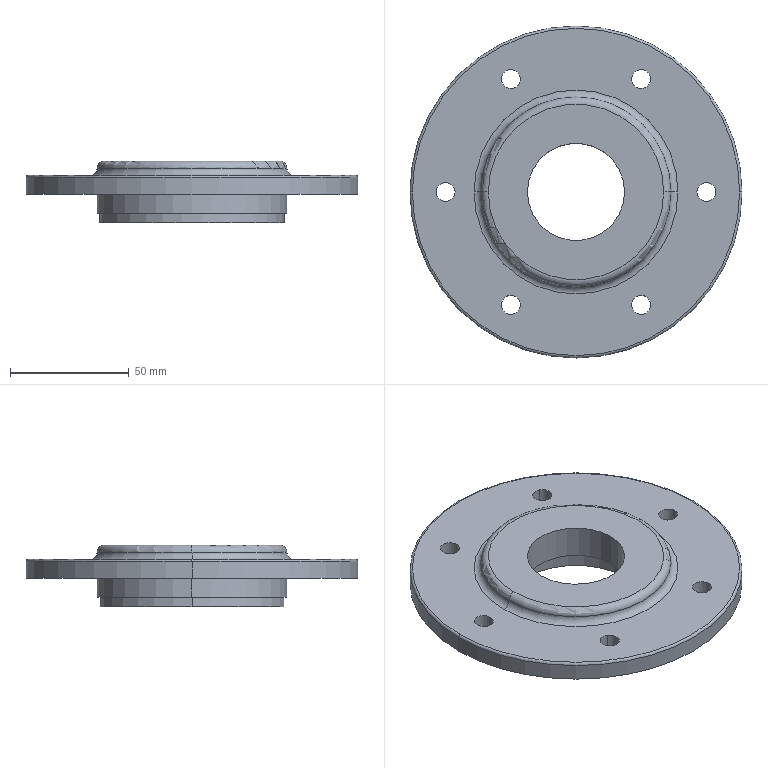Part | SolidWorks | features BaseBody 1 | 1 solid | 34 faces | box 140 x 140 x 26 mm | volume 157732 mm3 | cylinder 22 | torus 6 | plane 6 | commonest cylinder face diameters 8 x12 41 x2 60 x2 78 x2 80 x2 140 x2
STEP:
#1=CARTESIAN_POINT('',(-43.,0.,8.));
#2=VERTEX_POINT('',#1);
#3=CARTESIAN_POINT('',(43.,0.,8.));
#4=VERTEX_POINT('',#3);
#5=CARTESIAN_POINT('',(0.,0.,8.));
#6=DIRECTION('',(0.,0.,1.));
#7=DIRECTION('',(-1.,0.,0.));
#8=AXIS2_PLACEMENT_3D('',#5,#6,#7);
#9=CIRCLE('',#8,43.);
#10=EDGE_CURVE('',#2,#4,#9,.T.);
#11=ORIENTED_EDGE('',*,*,#10,.T.);
#12=CARTESIAN_POINT('',(40.,0.,11.));
#13=VERTEX_POINT('',#12);
#14=CARTESIAN_POINT('',(43.,0.,11.));
#15=DIRECTION('',(0.,1.,0.));
#16=DIRECTION('',(-1.,0.,0.));
#17=AXIS2_PLACEMENT_3D('',#14,#15,#16);
#18=CIRCLE('',#17,3.);
#19=EDGE_CURVE('',#4,#13,#18,.T.);
#20=ORIENTED_EDGE('',*,*,#19,.T.);
#21=CARTESIAN_POINT('',(-40.,0.,11.));
#22=VERTEX_POINT('',#21);
#23=CARTESIAN_POINT('',(0.,0.,11.));
#24=DIRECTION('',(0.,0.,1.));
#25=DIRECTION('',(-1.,0.,0.));
#26=AXIS2_PLACEMENT_3D('',#23,#24,#25);
#27=CIRCLE('',#26,40.);
#28=EDGE_CURVE('',#22,#13,#27,.T.);
#29=ORIENTED_EDGE('',*,*,#28,.F.);
#30=CARTESIAN_POINT('',(-43.,0.,11.));
#31=DIRECTION('',(0.,-1.,0.));
#32=DIRECTION('',(0.,0.,-1.));
#33=AXIS2_PLACEMENT_3D('',#30,#31,#32);
#34=CIRCLE('',#33,3.);
#35=EDGE_CURVE('',#2,#22,#34,.T.);
#36=ORIENTED_EDGE('',*,*,#35,.F.);
#37=EDGE_LOOP('',(#11,#20,#29,#36));
#38=FACE_OUTER_BOUND('',#37,.T.);
#39=CARTESIAN_POINT('',(0.,0.,11.));
#40=DIRECTION('',(0.,0.,-1.));
#41=DIRECTION('',(-1.,0.,0.));
#42=AXIS2_PLACEMENT_3D('',#39,#40,#41);
#43=TOROIDAL_SURFACE('',#42,43.,3.);
#44=ADVANCED_FACE('',(#38),#43,.F.);
#45=CARTESIAN_POINT('',(0.,0.,11.));
#46=DIRECTION('',(0.,0.,1.));
#47=DIRECTION('',(-1.,0.,0.));
#48=AXIS2_PLACEMENT_3D('',#45,#46,#47);
#49=CIRCLE('',#48,40.);
#50=EDGE_CURVE('',#13,#22,#49,.T.);
#51=ORIENTED_EDGE('',*,*,#50,.T.);
#52=CARTESIAN_POINT('',(-37.,0.,14.));
#53=VERTEX_POINT('',#52);
#54=CARTESIAN_POINT('',(-37.,0.,11.));
#55=DIRECTION('',(0.,1.,0.));
#56=DIRECTION('',(-1.,0.,0.));
#57=AXIS2_PLACEMENT_3D('',#54,#55,#56);
#58=CIRCLE('',#57,3.);
#59=EDGE_CURVE('',#22,#53,#58,.T.);
#60=ORIENTED_EDGE('',*,*,#59,.T.);
#61=CARTESIAN_POINT('',(37.,0.,14.));
#62=VERTEX_POINT('',#61);
#63=CARTESIAN_POINT('',(0.,0.,14.));
#64=DIRECTION('',(0.,0.,-1.));
#65=DIRECTION('',(-1.,0.,0.));
#66=AXIS2_PLACEMENT_3D('',#63,#64,#65);
#67=CIRCLE('',#66,37.);
#68=EDGE_CURVE('',#53,#62,#67,.T.);
#69=ORIENTED_EDGE('',*,*,#68,.T.);
#70=CARTESIAN_POINT('',(37.,0.,11.));
#71=DIRECTION('',(0.,-1.,0.));
#72=DIRECTION('',(0.,0.,-1.));
#73=AXIS2_PLACEMENT_3D('',#70,#71,#72);
#74=CIRCLE('',#73,3.);
#75=EDGE_CURVE('',#13,#62,#74,.T.);
#76=ORIENTED_EDGE('',*,*,#75,.F.);
#77=EDGE_LOOP('',(#51,#60,#69,#76));
#78=FACE_OUTER_BOUND('',#77,.T.);
#79=CARTESIAN_POINT('',(0.,0.,11.));
#80=DIRECTION('',(0.,0.,1.));
#81=DIRECTION('',(1.,0.,0.));
#82=AXIS2_PLACEMENT_3D('',#79,#80,#81);
#83=TOROIDAL_SURFACE('',#82,37.,3.);
#84=ADVANCED_FACE('',(#78),#83,.T.);
#85=CARTESIAN_POINT('',(20.5,0.,0.));
#86=VERTEX_POINT('',#85);
#87=CARTESIAN_POINT('',(-20.5,0.,0.));
#88=VERTEX_POINT('',#87);
#89=CARTESIAN_POINT('',(0.,0.,0.));
#90=DIRECTION('',(0.,0.,1.));
#91=DIRECTION('',(-1.,0.,0.));
#92=AXIS2_PLACEMENT_3D('',#89,#90,#91);
#93=CIRCLE('',#92,20.5);
#94=EDGE_CURVE('',#86,#88,#93,.T.);
#95=ORIENTED_EDGE('',*,*,#94,.F.);
#96=CARTESIAN_POINT('',(20.5,0.,14.));
#97=VERTEX_POINT('',#96);
#98=CARTESIAN_POINT('',(20.5,0.,14.));
#99=DIRECTION('',(0.,0.,1.));
#100=VECTOR('',#99,1000.);
#101=LINE('',#98,#100);
#102=EDGE_CURVE('',#86,#97,#101,.T.);
#103=ORIENTED_EDGE('',*,*,#102,.T.);
#104=CARTESIAN_POINT('',(-20.5,0.,14.));
#105=VERTEX_POINT('',#104);
#106=CARTESIAN_POINT('',(0.,0.,14.));
#107=DIRECTION('',(0.,0.,-1.));
#108=DIRECTION('',(-1.,0.,0.));
#109=AXIS2_PLACEMENT_3D('',#106,#107,#108);
#110=CIRCLE('',#109,20.5);
#111=EDGE_CURVE('',#105,#97,#110,.T.);
#112=ORIENTED_EDGE('',*,*,#111,.F.);
#113=CARTESIAN_POINT('',(-20.5,0.,14.));
#114=DIRECTION('',(0.,0.,1.));
#115=VECTOR('',#114,1000.);
#116=LINE('',#113,#115);
#117=EDGE_CURVE('',#88,#105,#116,.T.);
#118=ORIENTED_EDGE('',*,*,#117,.F.);
#119=EDGE_LOOP('',(#95,#103,#112,#118));
#120=FACE_OUTER_BOUND('',#119,.T.);
#121=CARTESIAN_POINT('',(0.,0.,14.));
#122=DIRECTION('',(0.,0.,1.));
#123=DIRECTION('',(-1.,0.,0.));
#124=AXIS2_PLACEMENT_3D('',#121,#122,#123);
#125=CYLINDRICAL_SURFACE('',#124,20.5);
#126=ADVANCED_FACE('',(#120),#125,.F.);
#127=CARTESIAN_POINT('',(-25.5,44.167,0.));
#128=VERTEX_POINT('',#127);
#129=CARTESIAN_POINT('',(-29.5,51.095,0.));
#130=VERTEX_POINT('',#129);
#131=CARTESIAN_POINT('',(-27.5,47.631,0.));
#132=DIRECTION('',(0.,0.,1.));
#133=DIRECTION('',(-0.5,0.866,0.));
#134=AXIS2_PLACEMENT_3D('',#131,#132,#133);
#135=CIRCLE('',#134,4.);
#136=EDGE_CURVE('',#128,#130,#135,.T.);
#137=ORIENTED_EDGE('',*,*,#136,.F.);
#138=CARTESIAN_POINT('',(-25.5,44.167,8.));
#139=VERTEX_POINT('',#138);
#140=CARTESIAN_POINT('',(-25.5,44.167,8.));
#141=DIRECTION('',(0.,0.,1.));
#142=VECTOR('',#141,1000.);
#143=LINE('',#140,#142);
#144=EDGE_CURVE('',#128,#139,#143,.T.);
#145=ORIENTED_EDGE('',*,*,#144,.T.);
#146=CARTESIAN_POINT('',(-29.5,51.095,8.));
#147=VERTEX_POINT('',#146);
#148=CARTESIAN_POINT('',(-27.5,47.631,8.));
#149=DIRECTION('',(0.,0.,-1.));
#150=DIRECTION('',(-0.5,0.866,0.));
#151=AXIS2_PLACEMENT_3D('',#148,#149,#150);
#152=CIRCLE('',#151,4.);
#153=EDGE_CURVE('',#147,#139,#152,.T.);
#154=ORIENTED_EDGE('',*,*,#153,.F.);
#155=CARTESIAN_POINT('',(-29.5,51.095,8.));
#156=DIRECTION('',(0.,0.,1.));
#157=VECTOR('',#156,1000.);
#158=LINE('',#155,#157);
#159=EDGE_CURVE('',#130,#147,#158,.T.);
#160=ORIENTED_EDGE('',*,*,#159,.F.);
#161=EDGE_LOOP('',(#137,#145,#154,#160));
#162=FACE_OUTER_BOUND('',#161,.T.);
#163=CARTESIAN_POINT('',(-27.5,47.631,8.));
#164=DIRECTION('',(0.,0.,1.));
#165=DIRECTION('',(-0.5,0.866,0.));
#166=AXIS2_PLACEMENT_3D('',#163,#164,#165);
#167=CYLINDRICAL_SURFACE('',#166,4.);
#168=ADVANCED_FACE('',(#162),#167,.F.);
#169=CARTESIAN_POINT('',(25.5,44.167,0.));
#170=VERTEX_POINT('',#169);
#171=CARTESIAN_POINT('',(29.5,51.095,0.));
#172=VERTEX_POINT('',#171);
#173=CARTESIAN_POINT('',(27.5,47.631,0.));
#174=DIRECTION('',(0.,0.,1.));
#175=DIRECTION('',(0.5,0.866,0.));
#176=AXIS2_PLACEMENT_3D('',#173,#174,#175);
#177=CIRCLE('',#176,4.);
#178=EDGE_CURVE('',#170,#172,#177,.T.);
#179=ORIENTED_EDGE('',*,*,#178,.F.);
#180=CARTESIAN_POINT('',(25.5,44.167,8.));
#181=VERTEX_POINT('',#180);
#182=CARTESIAN_POINT('',(25.5,44.167,8.));
#183=DIRECTION('',(0.,0.,1.));
#184=VECTOR('',#183,1000.);
#185=LINE('',#182,#184);
#186=EDGE_CURVE('',#170,#181,#185,.T.);
#187=ORIENTED_EDGE('',*,*,#186,.T.);
#188=CARTESIAN_POINT('',(29.5,51.095,8.));
#189=VERTEX_POINT('',#188);
#190=CARTESIAN_POINT('',(27.5,47.631,8.));
#191=DIRECTION('',(0.,0.,-1.));
#192=DIRECTION('',(0.5,0.866,0.));
#193=AXIS2_PLACEMENT_3D('',#190,#191,#192);
#194=CIRCLE('',#193,4.);
#195=EDGE_CURVE('',#189,#181,#194,.T.);
#196=ORIENTED_EDGE('',*,*,#195,.F.);
#197=CARTESIAN_POINT('',(29.5,51.095,8.));
#198=DIRECTION('',(0.,0.,1.));
#199=VECTOR('',#198,1000.);
#200=LINE('',#197,#199);
#201=EDGE_CURVE('',#172,#189,#200,.T.);
#202=ORIENTED_EDGE('',*,*,#201,.F.);
#203=EDGE_LOOP('',(#179,#187,#196,#202));
#204=FACE_OUTER_BOUND('',#203,.T.);
#205=CARTESIAN_POINT('',(27.5,47.631,8.));
#206=DIRECTION('',(0.,0.,1.));
#207=DIRECTION('',(0.5,0.866,0.));
#208=AXIS2_PLACEMENT_3D('',#205,#206,#207);
#209=CYLINDRICAL_SURFACE('',#208,4.);
#210=ADVANCED_FACE('',(#204),#209,.F.);
#211=CARTESIAN_POINT('',(51.,0.,0.));
#212=VERTEX_POINT('',#211);
#213=CARTESIAN_POINT('',(59.,0.,0.));
#214=VERTEX_POINT('',#213);
#215=CARTESIAN_POINT('',(55.,0.,0.));
#216=DIRECTION('',(0.,0.,1.));
#217=DIRECTION('',(1.,0.,0.));
#218=AXIS2_PLACEMENT_3D('',#215,#216,#217);
#219=CIRCLE('',#218,4.);
#220=EDGE_CURVE('',#212,#214,#219,.T.);
#221=ORIENTED_EDGE('',*,*,#220,.F.);
#222=CARTESIAN_POINT('',(51.,0.,8.));
#223=VERTEX_POINT('',#222);
#224=CARTESIAN_POINT('',(51.,0.,8.));
#225=DIRECTION('',(0.,0.,1.));
#226=VECTOR('',#225,1000.);
#227=LINE('',#224,#226);
#228=EDGE_CURVE('',#212,#223,#227,.T.);
#229=ORIENTED_EDGE('',*,*,#228,.T.);
#230=CARTESIAN_POINT('',(59.,0.,8.));
#231=VERTEX_POINT('',#230);
#232=CARTESIAN_POINT('',(55.,0.,8.));
#233=DIRECTION('',(0.,0.,-1.));
#234=DIRECTION('',(1.,0.,0.));
#235=AXIS2_PLACEMENT_3D('',#232,#233,#234);
#236=CIRCLE('',#235,4.);
#237=EDGE_CURVE('',#231,#223,#236,.T.);
#238=ORIENTED_EDGE('',*,*,#237,.F.);
#239=CARTESIAN_POINT('',(59.,0.,8.));
#240=DIRECTION('',(0.,0.,1.));
#241=VECTOR('',#240,1000.);
#242=LINE('',#239,#241);
#243=EDGE_CURVE('',#214,#231,#242,.T.);
#244=ORIENTED_EDGE('',*,*,#243,.F.);
#245=EDGE_LOOP('',(#221,#229,#238,#244));
#246=FACE_OUTER_BOUND('',#245,.T.);
#247=CARTESIAN_POINT('',(55.,0.,8.));
#248=DIRECTION('',(0.,0.,1.));
#249=DIRECTION('',(1.,0.,0.));
#250=AXIS2_PLACEMENT_3D('',#247,#248,#249);
#251=CYLINDRICAL_SURFACE('',#250,4.);
#252=ADVANCED_FACE('',(#246),#251,.F.);
#253=CARTESIAN_POINT('',(25.5,-44.167,0.));
#254=VERTEX_POINT('',#253);
#255=CARTESIAN_POINT('',(29.5,-51.095,0.));
#256=VERTEX_POINT('',#255);
#257=CARTESIAN_POINT('',(27.5,-47.631,0.));
#258=DIRECTION('',(0.,0.,1.));
#259=DIRECTION('',(0.5,-0.866,0.));
#260=AXIS2_PLACEMENT_3D('',#257,#258,#259);
#261=CIRCLE('',#260,4.);
#262=EDGE_CURVE('',#254,#256,#261,.T.);
#263=ORIENTED_EDGE('',*,*,#262,.F.);
#264=CARTESIAN_POINT('',(25.5,-44.167,8.));
#265=VERTEX_POINT('',#264);
#266=CARTESIAN_POINT('',(25.5,-44.167,8.));
#267=DIRECTION('',(0.,0.,1.));
#268=VECTOR('',#267,1000.);
#269=LINE('',#266,#268);
#270=EDGE_CURVE('',#254,#265,#269,.T.);
#271=ORIENTED_EDGE('',*,*,#270,.T.);
#272=CARTESIAN_POINT('',(29.5,-51.095,8.));
#273=VERTEX_POINT('',#272);
#274=CARTESIAN_POINT('',(27.5,-47.631,8.));
#275=DIRECTION('',(0.,0.,-1.));
#276=DIRECTION('',(0.5,-0.866,0.));
#277=AXIS2_PLACEMENT_3D('',#274,#275,#276);
#278=CIRCLE('',#277,4.);
#279=EDGE_CURVE('',#273,#265,#278,.T.);
#280=ORIENTED_EDGE('',*,*,#279,.F.);
#281=CARTESIAN_POINT('',(29.5,-51.095,8.));
#282=DIRECTION('',(0.,0.,1.));
#283=VECTOR('',#282,1000.);
#284=LINE('',#281,#283);
#285=EDGE_CURVE('',#256,#273,#284,.T.);
#286=ORIENTED_EDGE('',*,*,#285,.F.);
#287=EDGE_LOOP('',(#263,#271,#280,#286));
#288=FACE_OUTER_BOUND('',#287,.T.);
#289=CARTESIAN_POINT('',(27.5,-47.631,8.));
#290=DIRECTION('',(0.,0.,1.));
#291=DIRECTION('',(0.5,-0.866,0.));
#292=AXIS2_PLACEMENT_3D('',#289,#290,#291);
#293=CYLINDRICAL_SURFACE('',#292,4.);
#294=ADVANCED_FACE('',(#288),#293,.F.);
#295=CARTESIAN_POINT('',(-25.5,-44.167,0.));
#296=VERTEX_POINT('',#295);
#297=CARTESIAN_POINT('',(-29.5,-51.095,0.));
#298=VERTEX_POINT('',#297);
#299=CARTESIAN_POINT('',(-27.5,-47.631,0.));
#300=DIRECTION('',(0.,0.,1.));
#301=DIRECTION('',(-0.5,-0.866,0.));
#302=AXIS2_PLACEMENT_3D('',#299,#300,#301);
#303=CIRCLE('',#302,4.);
#304=EDGE_CURVE('',#296,#298,#303,.T.);
#305=ORIENTED_EDGE('',*,*,#304,.F.);
#306=CARTESIAN_POINT('',(-25.5,-44.167,8.));
#307=VERTEX_POINT('',#306);
#308=CARTESIAN_POINT('',(-25.5,-44.167,8.));
#309=DIRECTION('',(0.,0.,1.));
#310=VECTOR('',#309,1000.);
#311=LINE('',#308,#310);
#312=EDGE_CURVE('',#296,#307,#311,.T.);
#313=ORIENTED_EDGE('',*,*,#312,.T.);
#314=CARTESIAN_POINT('',(-29.5,-51.095,8.));
#315=VERTEX_POINT('',#314);
#316=CARTESIAN_POINT('',(-27.5,-47.631,8.));
#317=DIRECTION('',(0.,0.,-1.));
#318=DIRECTION('',(-0.5,-0.866,0.));
#319=AXIS2_PLACEMENT_3D('',#316,#317,#318);
#320=CIRCLE('',#319,4.);
#321=EDGE_CURVE('',#315,#307,#320,.T.);
#322=ORIENTED_EDGE('',*,*,#321,.F.);
#323=CARTESIAN_POINT('',(-29.5,-51.095,8.));
#324=DIRECTION('',(0.,0.,1.));
#325=VECTOR('',#324,1000.);
#326=LINE('',#323,#325);
#327=EDGE_CURVE('',#298,#315,#326,.T.);
#328=ORIENTED_EDGE('',*,*,#327,.F.);
#329=EDGE_LOOP('',(#305,#313,#322,#328));
#330=FACE_OUTER_BOUND('',#329,.T.);
#331=CARTESIAN_POINT('',(-27.5,-47.631,8.));
#332=DIRECTION('',(0.,0.,1.));
#333=DIRECTION('',(-0.5,-0.866,0.));
#334=AXIS2_PLACEMENT_3D('',#331,#332,#333);
#335=CYLINDRICAL_SURFACE('',#334,4.);
#336=ADVANCED_FACE('',(#330),#335,.F.);
#337=CARTESIAN_POINT('',(-51.,0.,0.));
#338=VERTEX_POINT('',#337);
#339=CARTESIAN_POINT('',(-59.,0.,0.));
#340=VERTEX_POINT('',#339);
#341=CARTESIAN_POINT('',(-55.,0.,0.));
#342=DIRECTION('',(0.,0.,1.));
#343=DIRECTION('',(-1.,0.,0.));
#344=AXIS2_PLACEMENT_3D('',#341,#342,#343);
#345=CIRCLE('',#344,4.);
#346=EDGE_CURVE('',#338,#340,#345,.T.);
#347=ORIENTED_EDGE('',*,*,#346,.F.);
#348=CARTESIAN_POINT('',(-51.,0.,8.));
#349=VERTEX_POINT('',#348);
#350=CARTESIAN_POINT('',(-51.,0.,8.));
#351=DIRECTION('',(0.,0.,1.));
#352=VECTOR('',#351,1000.);
#353=LINE('',#350,#352);
#354=EDGE_CURVE('',#338,#349,#353,.T.);
#355=ORIENTED_EDGE('',*,*,#354,.T.);
#356=CARTESIAN_POINT('',(-59.,0.,8.));
#357=VERTEX_POINT('',#356);
#358=CARTESIAN_POINT('',(-55.,0.,8.));
#359=DIRECTION('',(0.,0.,-1.));
#360=DIRECTION('',(-1.,0.,0.));
#361=AXIS2_PLACEMENT_3D('',#358,#359,#360);
#362=CIRCLE('',#361,4.);
#363=EDGE_CURVE('',#357,#349,#362,.T.);
#364=ORIENTED_EDGE('',*,*,#363,.F.);
#365=CARTESIAN_POINT('',(-59.,0.,8.));
#366=DIRECTION('',(0.,0.,1.));
#367=VECTOR('',#366,1000.);
#368=LINE('',#365,#367);
#369=EDGE_CURVE('',#340,#357,#368,.T.);
#370=ORIENTED_EDGE('',*,*,#369,.F.);
#371=EDGE_LOOP('',(#347,#355,#364,#370));
#372=FACE_OUTER_BOUND('',#371,.T.);
#373=CARTESIAN_POINT('',(-55.,0.,8.));
#374=DIRECTION('',(0.,0.,1.));
#375=DIRECTION('',(-1.,0.,0.));
#376=AXIS2_PLACEMENT_3D('',#373,#374,#375);
#377=CYLINDRICAL_SURFACE('',#376,4.);
#378=ADVANCED_FACE('',(#372),#377,.F.);
#379=CARTESIAN_POINT('',(70.,0.,7.));
#380=VERTEX_POINT('',#379);
#381=CARTESIAN_POINT('',(-70.,0.,7.));
#382=VERTEX_POINT('',#381);
#383=CARTESIAN_POINT('',(0.,0.,7.));
#384=DIRECTION('',(0.,0.,1.));
#385=DIRECTION('',(-1.,0.,0.));
#386=AXIS2_PLACEMENT_3D('',#383,#384,#385);
#387=CIRCLE('',#386,70.);
#388=EDGE_CURVE('',#380,#382,#387,.T.);
#389=ORIENTED_EDGE('',*,*,#388,.T.);
#390=CARTESIAN_POINT('',(-69.,0.,8.));
#391=VERTEX_POINT('',#390);
#392=CARTESIAN_POINT('',(-69.,0.,7.));
#393=DIRECTION('',(0.,1.,0.));
#394=DIRECTION('',(-1.,0.,0.));
#395=AXIS2_PLACEMENT_3D('',#392,#393,#394);
#396=CIRCLE('',#395,1.);
#397=EDGE_CURVE('',#382,#391,#396,.T.);
#398=ORIENTED_EDGE('',*,*,#397,.T.);
#399=CARTESIAN_POINT('',(69.,0.,8.));
#400=VERTEX_POINT('',#399);
#401=CARTESIAN_POINT('',(0.,0.,8.));
#402=DIRECTION('',(0.,0.,-1.));
#403=DIRECTION('',(-1.,0.,0.));
#404=AXIS2_PLACEMENT_3D('',#401,#402,#403);
#405=CIRCLE('',#404,69.);
#406=EDGE_CURVE('',#391,#400,#405,.T.);
#407=ORIENTED_EDGE('',*,*,#406,.T.);
#408=CARTESIAN_POINT('',(69.,0.,7.));
#409=DIRECTION('',(0.,-1.,0.));
#410=DIRECTION('',(0.,0.,-1.));
#411=AXIS2_PLACEMENT_3D('',#408,#409,#410);
#412=CIRCLE('',#411,1.);
#413=EDGE_CURVE('',#380,#400,#412,.T.);
#414=ORIENTED_EDGE('',*,*,#413,.F.);
#415=EDGE_LOOP('',(#389,#398,#407,#414));
#416=FACE_OUTER_BOUND('',#415,.T.);
#417=CARTESIAN_POINT('',(0.,0.,7.));
#418=DIRECTION('',(0.,0.,1.));
#419=DIRECTION('',(1.,0.,0.));
#420=AXIS2_PLACEMENT_3D('',#417,#418,#419);
#421=TOROIDAL_SURFACE('',#420,69.,1.);
#422=ADVANCED_FACE('',(#416),#421,.T.);
#423=ORIENTED_EDGE('',*,*,#388,.F.);
#424=CARTESIAN_POINT('',(70.,0.,0.));
#425=VERTEX_POINT('',#424);
#426=CARTESIAN_POINT('',(70.,0.,0.));
#427=DIRECTION('',(0.,0.,-1.));
#428=VECTOR('',#427,1000.);
#429=LINE('',#426,#428);
#430=EDGE_CURVE('',#380,#425,#429,.T.);
#431=ORIENTED_EDGE('',*,*,#430,.T.);
#432=CARTESIAN_POINT('',(-70.,0.,0.));
#433=VERTEX_POINT('',#432);
#434=CARTESIAN_POINT('',(0.,0.,0.));
#435=DIRECTION('',(0.,0.,-1.));
#436=DIRECTION('',(-1.,0.,0.));
#437=AXIS2_PLACEMENT_3D('',#434,#435,#436);
#438=CIRCLE('',#437,70.);
#439=EDGE_CURVE('',#433,#425,#438,.T.);
#440=ORIENTED_EDGE('',*,*,#439,.F.);
#441=CARTESIAN_POINT('',(-70.,0.,0.));
#442=DIRECTION('',(0.,0.,-1.));
#443=VECTOR('',#442,1000.);
#444=LINE('',#441,#443);
#445=EDGE_CURVE('',#382,#433,#444,.T.);
#446=ORIENTED_EDGE('',*,*,#445,.F.);
#447=EDGE_LOOP('',(#423,#431,#440,#446));
#448=FACE_OUTER_BOUND('',#447,.T.);
#449=CARTESIAN_POINT('',(0.,0.,0.));
#450=DIRECTION('',(0.,0.,-1.));
#451=DIRECTION('',(-1.,0.,0.));
#452=AXIS2_PLACEMENT_3D('',#449,#450,#451);
#453=CYLINDRICAL_SURFACE('',#452,70.);
#454=ADVANCED_FACE('',(#448),#453,.T.);
#455=CARTESIAN_POINT('',(39.,0.,-8.));
#456=VERTEX_POINT('',#455);
#457=CARTESIAN_POINT('',(-39.,0.,-8.));
#458=VERTEX_POINT('',#457);
#459=CARTESIAN_POINT('',(0.,0.,-8.));
#460=DIRECTION('',(0.,0.,-1.));
#461=DIRECTION('',(1.,0.,0.));
#462=AXIS2_PLACEMENT_3D('',#459,#460,#461);
#463=CIRCLE('',#462,39.);
#464=EDGE_CURVE('',#456,#458,#463,.T.);
#465=ORIENTED_EDGE('',*,*,#464,.T.);
#466=CARTESIAN_POINT('',(-39.,0.,-12.));
#467=VERTEX_POINT('',#466);
#468=CARTESIAN_POINT('',(-39.,0.,-12.));
#469=DIRECTION('',(0.,0.,-1.));
#470=VECTOR('',#469,1000.);
#471=LINE('',#468,#470);
#472=EDGE_CURVE('',#458,#467,#471,.T.);
#473=ORIENTED_EDGE('',*,*,#472,.T.);
#474=CARTESIAN_POINT('',(39.,0.,-12.));
#475=VERTEX_POINT('',#474);
#476=CARTESIAN_POINT('',(0.,0.,-12.));
#477=DIRECTION('',(0.,0.,-1.));
#478=DIRECTION('',(1.,0.,0.));
#479=AXIS2_PLACEMENT_3D('',#476,#477,#478);
#480=CIRCLE('',#479,39.);
#481=EDGE_CURVE('',#475,#467,#480,.T.);
#482=ORIENTED_EDGE('',*,*,#481,.F.);
#483=CARTESIAN_POINT('',(39.,0.,-12.));
#484=DIRECTION('',(0.,0.,-1.));
#485=VECTOR('',#484,1000.);
#486=LINE('',#483,#485);
#487=EDGE_CURVE('',#456,#475,#486,.T.);
#488=ORIENTED_EDGE('',*,*,#487,.F.);
#489=EDGE_LOOP('',(#465,#473,#482,#488));
#490=FACE_OUTER_BOUND('',#489,.T.);
#491=CARTESIAN_POINT('',(0.,0.,-12.));
#492=DIRECTION('',(0.,0.,-1.));
#493=DIRECTION('',(1.,0.,0.));
#494=AXIS2_PLACEMENT_3D('',#491,#492,#493);
#495=CYLINDRICAL_SURFACE('',#494,39.);
#496=ADVANCED_FACE('',(#490),#495,.T.);
#497=CARTESIAN_POINT('',(-30.,0.,-12.));
#498=VERTEX_POINT('',#497);
#499=CARTESIAN_POINT('',(30.,0.,-12.));
#500=VERTEX_POINT('',#499);
#501=CARTESIAN_POINT('',(0.,0.,-12.));
#502=DIRECTION('',(0.,0.,1.));
#503=DIRECTION('',(1.,0.,0.));
#504=AXIS2_PLACEMENT_3D('',#501,#502,#503);
#505=CIRCLE('',#504,30.);
#506=EDGE_CURVE('',#498,#500,#505,.T.);
#507=ORIENTED_EDGE('',*,*,#506,.F.);
#508=CARTESIAN_POINT('',(-30.,0.,0.));
#509=VERTEX_POINT('',#508);
#510=CARTESIAN_POINT('',(-30.,0.,0.));
#511=DIRECTION('',(0.,0.,1.));
#512=VECTOR('',#511,1000.);
#513=LINE('',#510,#512);
#514=EDGE_CURVE('',#498,#509,#513,.T.);
#515=ORIENTED_EDGE('',*,*,#514,.T.);
#516=CARTESIAN_POINT('',(30.,0.,0.));
#517=VERTEX_POINT('',#516);
#518=CARTESIAN_POINT('',(0.,0.,0.));
#519=DIRECTION('',(0.,0.,-1.));
#520=DIRECTION('',(1.,0.,0.));
#521=AXIS2_PLACEMENT_3D('',#518,#519,#520);
#522=CIRCLE('',#521,30.);
#523=EDGE_CURVE('',#517,#509,#522,.T.);
#524=ORIENTED_EDGE('',*,*,#523,.F.);
#525=CARTESIAN_POINT('',(30.,0.,0.));
#526=DIRECTION('',(0.,0.,1.));
#527=VECTOR('',#526,1000.);
#528=LINE('',#525,#527);
#529=EDGE_CURVE('',#500,#517,#528,.T.);
#530=ORIENTED_EDGE('',*,*,#529,.F.);
#531=EDGE_LOOP('',(#507,#515,#524,#530));
#532=FACE_OUTER_BOUND('',#531,.T.);
#533=CARTESIAN_POINT('',(0.,0.,0.));
#534=DIRECTION('',(0.,0.,1.));
#535=DIRECTION('',(1.,0.,0.));
#536=AXIS2_PLACEMENT_3D('',#533,#534,#535);
#537=CYLINDRICAL_SURFACE('',#536,30.);
#538=ADVANCED_FACE('',(#532),#537,.F.);
#539=CARTESIAN_POINT('',(40.,0.,-8.));
#540=VERTEX_POINT('',#539);
#541=CARTESIAN_POINT('',(-40.,0.,-8.));
#542=VERTEX_POINT('',#541);
#543=CARTESIAN_POINT('',(0.,0.,-8.));
#544=DIRECTION('',(0.,0.,1.));
#545=DIRECTION('',(1.,0.,0.));
#546=AXIS2_PLACEMENT_3D('',#543,#544,#545);
#547=CIRCLE('',#546,40.);
#548=EDGE_CURVE('',#540,#542,#547,.T.);
#549=ORIENTED_EDGE('',*,*,#548,.T.);
#550=CARTESIAN_POINT('',(-40.,0.,0.));
#551=VERTEX_POINT('',#550);
#552=CARTESIAN_POINT('',(-40.,0.,0.));
#553=DIRECTION('',(0.,0.,1.));
#554=VECTOR('',#553,1000.);
#555=LINE('',#552,#554);
#556=EDGE_CURVE('',#542,#551,#555,.T.);
#557=ORIENTED_EDGE('',*,*,#556,.T.);
#558=CARTESIAN_POINT('',(40.,0.,0.));
#559=VERTEX_POINT('',#558);
#560=CARTESIAN_POINT('',(0.,0.,0.));
#561=DIRECTION('',(0.,0.,1.));
#562=DIRECTION('',(1.,0.,0.));
#563=AXIS2_PLACEMENT_3D('',#560,#561,#562);
#564=CIRCLE('',#563,40.);
#565=EDGE_CURVE('',#559,#551,#564,.T.);
#566=ORIENTED_EDGE('',*,*,#565,.F.);
#567=CARTESIAN_POINT('',(40.,0.,0.));
#568=DIRECTION('',(0.,0.,1.));
#569=VECTOR('',#568,1000.);
#570=LINE('',#567,#569);
#571=EDGE_CURVE('',#540,#559,#570,.T.);
#572=ORIENTED_EDGE('',*,*,#571,.F.);
#573=EDGE_LOOP('',(#549,#557,#566,#572));
#574=FACE_OUTER_BOUND('',#573,.T.);
#575=CARTESIAN_POINT('',(0.,0.,0.));
#576=DIRECTION('',(0.,0.,1.));
#577=DIRECTION('',(1.,0.,0.));
#578=AXIS2_PLACEMENT_3D('',#575,#576,#577);
#579=CYLINDRICAL_SURFACE('',#578,40.);
#580=ADVANCED_FACE('',(#574),#579,.T.);
#581=ORIENTED_EDGE('',*,*,#363,.T.);
#582=CARTESIAN_POINT('',(-55.,0.,8.));
#583=DIRECTION('',(0.,0.,-1.));
#584=DIRECTION('',(-1.,0.,0.));
#585=AXIS2_PLACEMENT_3D('',#582,#583,#584);
#586=CIRCLE('',#585,4.);
#587=EDGE_CURVE('',#349,#357,#586,.T.);
#588=ORIENTED_EDGE('',*,*,#587,.T.);
#589=EDGE_LOOP('',(#581,#588));
#590=FACE_BOUND('',#589,.T.);
#591=ORIENTED_EDGE('',*,*,#321,.T.);
#592=CARTESIAN_POINT('',(-27.5,-47.631,8.));
#593=DIRECTION('',(0.,0.,-1.));
#594=DIRECTION('',(-0.5,-0.866,0.));
#595=AXIS2_PLACEMENT_3D('',#592,#593,#594);
#596=CIRCLE('',#595,4.);
#597=EDGE_CURVE('',#307,#315,#596,.T.);
#598=ORIENTED_EDGE('',*,*,#597,.T.);
#599=EDGE_LOOP('',(#591,#598));
#600=FACE_BOUND('',#599,.T.);
#601=ORIENTED_EDGE('',*,*,#279,.T.);
#602=CARTESIAN_POINT('',(27.5,-47.631,8.));
#603=DIRECTION('',(0.,0.,-1.));
#604=DIRECTION('',(0.5,-0.866,0.));
#605=AXIS2_PLACEMENT_3D('',#602,#603,#604);
#606=CIRCLE('',#605,4.);
#607=EDGE_CURVE('',#265,#273,#606,.T.);
#608=ORIENTED_EDGE('',*,*,#607,.T.);
#609=EDGE_LOOP('',(#601,#608));
#610=FACE_BOUND('',#609,.T.);
#611=ORIENTED_EDGE('',*,*,#237,.T.);
#612=CARTESIAN_POINT('',(55.,0.,8.));
#613=DIRECTION('',(0.,0.,-1.));
#614=DIRECTION('',(1.,0.,0.));
#615=AXIS2_PLACEMENT_3D('',#612,#613,#614);
#616=CIRCLE('',#615,4.);
#617=EDGE_CURVE('',#223,#231,#616,.T.);
#618=ORIENTED_EDGE('',*,*,#617,.T.);
#619=EDGE_LOOP('',(#611,#618));
#620=FACE_BOUND('',#619,.T.);
#621=ORIENTED_EDGE('',*,*,#195,.T.);
#622=CARTESIAN_POINT('',(27.5,47.631,8.));
#623=DIRECTION('',(0.,0.,-1.));
#624=DIRECTION('',(0.5,0.866,0.));
#625=AXIS2_PLACEMENT_3D('',#622,#623,#624);
#626=CIRCLE('',#625,4.);
#627=EDGE_CURVE('',#181,#189,#626,.T.);
#628=ORIENTED_EDGE('',*,*,#627,.T.);
#629=EDGE_LOOP('',(#621,#628));
#630=FACE_BOUND('',#629,.T.);
#631=ORIENTED_EDGE('',*,*,#153,.T.);
#632=CARTESIAN_POINT('',(-27.5,47.631,8.));
#633=DIRECTION('',(0.,0.,-1.));
#634=DIRECTION('',(-0.5,0.866,0.));
#635=AXIS2_PLACEMENT_3D('',#632,#633,#634);
#636=CIRCLE('',#635,4.);
#637=EDGE_CURVE('',#139,#147,#636,.T.);
#638=ORIENTED_EDGE('',*,*,#637,.T.);
#639=EDGE_LOOP('',(#631,#638));
#640=FACE_BOUND('',#639,.T.);
#641=ORIENTED_EDGE('',*,*,#10,.F.);
#642=CARTESIAN_POINT('',(0.,0.,8.));
#643=DIRECTION('',(0.,0.,1.));
#644=DIRECTION('',(-1.,0.,0.));
#645=AXIS2_PLACEMENT_3D('',#642,#643,#644);
#646=CIRCLE('',#645,43.);
#647=EDGE_CURVE('',#4,#2,#646,.T.);
#648=ORIENTED_EDGE('',*,*,#647,.F.);
#649=EDGE_LOOP('',(#641,#648));
#650=FACE_BOUND('',#649,.T.);
#651=CARTESIAN_POINT('',(0.,0.,8.));
#652=DIRECTION('',(0.,0.,-1.));
#653=DIRECTION('',(-1.,0.,0.));
#654=AXIS2_PLACEMENT_3D('',#651,#652,#653);
#655=CIRCLE('',#654,69.);
#656=EDGE_CURVE('',#400,#391,#655,.T.);
#657=ORIENTED_EDGE('',*,*,#656,.F.);
#658=ORIENTED_EDGE('',*,*,#406,.F.);
#659=EDGE_LOOP('',(#657,#658));
#660=FACE_OUTER_BOUND('',#659,.T.);
#661=CARTESIAN_POINT('',(0.,0.,8.));
#662=DIRECTION('',(0.,0.,1.));
#663=DIRECTION('',(1.,0.,0.));
#664=AXIS2_PLACEMENT_3D('',#661,#662,#663);
#665=PLANE('',#664);
#666=ADVANCED_FACE('',(#590,#600,#610,#620,#630,#640,#650,#660),#665,.T.);
#667=ORIENTED_EDGE('',*,*,#111,.T.);
#668=CARTESIAN_POINT('',(0.,0.,14.));
#669=DIRECTION('',(0.,0.,-1.));
#670=DIRECTION('',(-1.,0.,0.));
#671=AXIS2_PLACEMENT_3D('',#668,#669,#670);
#672=CIRCLE('',#671,20.5);
#673=EDGE_CURVE('',#97,#105,#672,.T.);
#674=ORIENTED_EDGE('',*,*,#673,.T.);
#675=EDGE_LOOP('',(#667,#674));
#676=FACE_BOUND('',#675,.T.);
#677=CARTESIAN_POINT('',(0.,0.,14.));
#678=DIRECTION('',(0.,0.,-1.));
#679=DIRECTION('',(-1.,0.,0.));
#680=AXIS2_PLACEMENT_3D('',#677,#678,#679);
#681=CIRCLE('',#680,37.);
#682=EDGE_CURVE('',#62,#53,#681,.T.);
#683=ORIENTED_EDGE('',*,*,#682,.F.);
#684=ORIENTED_EDGE('',*,*,#68,.F.);
#685=EDGE_LOOP('',(#683,#684));
#686=FACE_OUTER_BOUND('',#685,.T.);
#687=CARTESIAN_POINT('',(0.,0.,14.));
#688=DIRECTION('',(0.,0.,1.));
#689=DIRECTION('',(1.,0.,0.));
#690=AXIS2_PLACEMENT_3D('',#687,#688,#689);
#691=PLANE('',#690);
#692=ADVANCED_FACE('',(#676,#686),#691,.T.);
#693=ORIENTED_EDGE('',*,*,#464,.F.);
#694=CARTESIAN_POINT('',(0.,0.,-8.));
#695=DIRECTION('',(0.,0.,-1.));
#696=DIRECTION('',(1.,0.,0.));
#697=AXIS2_PLACEMENT_3D('',#694,#695,#696);
#698=CIRCLE('',#697,39.);
#699=EDGE_CURVE('',#458,#456,#698,.T.);
#700=ORIENTED_EDGE('',*,*,#699,.F.);
#701=EDGE_LOOP('',(#693,#700));
#702=FACE_BOUND('',#701,.T.);
#703=ORIENTED_EDGE('',*,*,#548,.F.);
#704=CARTESIAN_POINT('',(0.,0.,-8.));
#705=DIRECTION('',(0.,0.,1.));
#706=DIRECTION('',(1.,0.,0.));
#707=AXIS2_PLACEMENT_3D('',#704,#705,#706);
#708=CIRCLE('',#707,40.);
#709=EDGE_CURVE('',#542,#540,#708,.T.);
#710=ORIENTED_EDGE('',*,*,#709,.F.);
#711=EDGE_LOOP('',(#703,#710));
#712=FACE_OUTER_BOUND('',#711,.T.);
#713=CARTESIAN_POINT('',(0.,0.,-8.));
#714=DIRECTION('',(0.,0.,1.));
#715=DIRECTION('',(1.,0.,0.));
#716=AXIS2_PLACEMENT_3D('',#713,#714,#715);
#717=PLANE('',#716);
#718=ADVANCED_FACE('',(#702,#712),#717,.F.);
#719=CARTESIAN_POINT('',(0.,0.,-12.));
#720=DIRECTION('',(0.,0.,1.));
#721=DIRECTION('',(1.,0.,0.));
#722=AXIS2_PLACEMENT_3D('',#719,#720,#721);
#723=CIRCLE('',#722,30.);
#724=EDGE_CURVE('',#500,#498,#723,.T.);
#725=ORIENTED_EDGE('',*,*,#724,.T.);
#726=ORIENTED_EDGE('',*,*,#506,.T.);
#727=EDGE_LOOP('',(#725,#726));
#728=FACE_BOUND('',#727,.T.);
#729=ORIENTED_EDGE('',*,*,#481,.T.);
#730=CARTESIAN_POINT('',(0.,0.,-12.));
#731=DIRECTION('',(0.,0.,-1.));
#732=DIRECTION('',(1.,0.,0.));
#733=AXIS2_PLACEMENT_3D('',#730,#731,#732);
#734=CIRCLE('',#733,39.);
#735=EDGE_CURVE('',#467,#475,#734,.T.);
#736=ORIENTED_EDGE('',*,*,#735,.T.);
#737=EDGE_LOOP('',(#729,#736));
#738=FACE_OUTER_BOUND('',#737,.T.);
#739=CARTESIAN_POINT('',(0.,0.,-12.));
#740=DIRECTION('',(0.,0.,1.));
#741=DIRECTION('',(1.,0.,0.));
#742=AXIS2_PLACEMENT_3D('',#739,#740,#741);
#743=PLANE('',#742);
#744=ADVANCED_FACE('',(#728,#738),#743,.F.);
#745=CARTESIAN_POINT('',(-27.5,47.631,0.));
#746=DIRECTION('',(0.,0.,1.));
#747=DIRECTION('',(-0.5,0.866,0.));
#748=AXIS2_PLACEMENT_3D('',#745,#746,#747);
#749=CIRCLE('',#748,4.);
#750=EDGE_CURVE('',#130,#128,#749,.T.);
#751=ORIENTED_EDGE('',*,*,#750,.T.);
#752=ORIENTED_EDGE('',*,*,#136,.T.);
#753=EDGE_LOOP('',(#751,#752));
#754=FACE_BOUND('',#753,.T.);
#755=CARTESIAN_POINT('',(27.5,47.631,0.));
#756=DIRECTION('',(0.,0.,1.));
#757=DIRECTION('',(0.5,0.866,0.));
#758=AXIS2_PLACEMENT_3D('',#755,#756,#757);
#759=CIRCLE('',#758,4.);
#760=EDGE_CURVE('',#172,#170,#759,.T.);
#761=ORIENTED_EDGE('',*,*,#760,.T.);
#762=ORIENTED_EDGE('',*,*,#178,.T.);
#763=EDGE_LOOP('',(#761,#762));
#764=FACE_BOUND('',#763,.T.);
#765=CARTESIAN_POINT('',(55.,0.,0.));
#766=DIRECTION('',(0.,0.,1.));
#767=DIRECTION('',(1.,0.,0.));
#768=AXIS2_PLACEMENT_3D('',#765,#766,#767);
#769=CIRCLE('',#768,4.);
#770=EDGE_CURVE('',#214,#212,#769,.T.);
#771=ORIENTED_EDGE('',*,*,#770,.T.);
#772=ORIENTED_EDGE('',*,*,#220,.T.);
#773=EDGE_LOOP('',(#771,#772));
#774=FACE_BOUND('',#773,.T.);
#775=CARTESIAN_POINT('',(27.5,-47.631,0.));
#776=DIRECTION('',(0.,0.,1.));
#777=DIRECTION('',(0.5,-0.866,0.));
#778=AXIS2_PLACEMENT_3D('',#775,#776,#777);
#779=CIRCLE('',#778,4.);
#780=EDGE_CURVE('',#256,#254,#779,.T.);
#781=ORIENTED_EDGE('',*,*,#780,.T.);
#782=ORIENTED_EDGE('',*,*,#262,.T.);
#783=EDGE_LOOP('',(#781,#782));
#784=FACE_BOUND('',#783,.T.);
#785=CARTESIAN_POINT('',(-27.5,-47.631,0.));
#786=DIRECTION('',(0.,0.,1.));
#787=DIRECTION('',(-0.5,-0.866,0.));
#788=AXIS2_PLACEMENT_3D('',#785,#786,#787);
#789=CIRCLE('',#788,4.);
#790=EDGE_CURVE('',#298,#296,#789,.T.);
#791=ORIENTED_EDGE('',*,*,#790,.T.);
#792=ORIENTED_EDGE('',*,*,#304,.T.);
#793=EDGE_LOOP('',(#791,#792));
#794=FACE_BOUND('',#793,.T.);
#795=CARTESIAN_POINT('',(-55.,0.,0.));
#796=DIRECTION('',(0.,0.,1.));
#797=DIRECTION('',(-1.,0.,0.));
#798=AXIS2_PLACEMENT_3D('',#795,#796,#797);
#799=CIRCLE('',#798,4.);
#800=EDGE_CURVE('',#340,#338,#799,.T.);
#801=ORIENTED_EDGE('',*,*,#800,.T.);
#802=ORIENTED_EDGE('',*,*,#346,.T.);
#803=EDGE_LOOP('',(#801,#802));
#804=FACE_BOUND('',#803,.T.);
#805=ORIENTED_EDGE('',*,*,#565,.T.);
#806=CARTESIAN_POINT('',(0.,0.,0.));
#807=DIRECTION('',(0.,0.,1.));
#808=DIRECTION('',(1.,0.,0.));
#809=AXIS2_PLACEMENT_3D('',#806,#807,#808);
#810=CIRCLE('',#809,40.);
#811=EDGE_CURVE('',#551,#559,#810,.T.);
#812=ORIENTED_EDGE('',*,*,#811,.T.);
#813=EDGE_LOOP('',(#805,#812));
#814=FACE_BOUND('',#813,.T.);
#815=ORIENTED_EDGE('',*,*,#439,.T.);
#816=CARTESIAN_POINT('',(0.,0.,0.));
#817=DIRECTION('',(0.,0.,-1.));
#818=DIRECTION('',(-1.,0.,0.));
#819=AXIS2_PLACEMENT_3D('',#816,#817,#818);
#820=CIRCLE('',#819,70.);
#821=EDGE_CURVE('',#425,#433,#820,.T.);
#822=ORIENTED_EDGE('',*,*,#821,.T.);
#823=EDGE_LOOP('',(#815,#822));
#824=FACE_OUTER_BOUND('',#823,.T.);
#825=CARTESIAN_POINT('',(0.,0.,0.));
#826=DIRECTION('',(0.,0.,1.));
#827=DIRECTION('',(1.,0.,0.));
#828=AXIS2_PLACEMENT_3D('',#825,#826,#827);
#829=PLANE('',#828);
#830=ADVANCED_FACE('',(#754,#764,#774,#784,#794,#804,#814,#824),#829,.F.);
#831=CARTESIAN_POINT('',(0.,0.,0.));
#832=DIRECTION('',(0.,0.,1.));
#833=DIRECTION('',(-1.,0.,0.));
#834=AXIS2_PLACEMENT_3D('',#831,#832,#833);
#835=CIRCLE('',#834,20.5);
#836=EDGE_CURVE('',#88,#86,#835,.T.);
#837=ORIENTED_EDGE('',*,*,#836,.T.);
#838=ORIENTED_EDGE('',*,*,#94,.T.);
#839=EDGE_LOOP('',(#837,#838));
#840=FACE_BOUND('',#839,.T.);
#841=ORIENTED_EDGE('',*,*,#523,.T.);
#842=CARTESIAN_POINT('',(0.,0.,0.));
#843=DIRECTION('',(0.,0.,-1.));
#844=DIRECTION('',(1.,0.,0.));
#845=AXIS2_PLACEMENT_3D('',#842,#843,#844);
#846=CIRCLE('',#845,30.);
#847=EDGE_CURVE('',#509,#517,#846,.T.);
#848=ORIENTED_EDGE('',*,*,#847,.T.);
#849=EDGE_LOOP('',(#841,#848));
#850=FACE_OUTER_BOUND('',#849,.T.);
#851=CARTESIAN_POINT('',(0.,0.,0.));
#852=DIRECTION('',(0.,0.,1.));
#853=DIRECTION('',(1.,0.,0.));
#854=AXIS2_PLACEMENT_3D('',#851,#852,#853);
#855=PLANE('',#854);
#856=ADVANCED_FACE('',(#840,#850),#855,.F.);
#857=ORIENTED_EDGE('',*,*,#556,.F.);
#858=ORIENTED_EDGE('',*,*,#709,.T.);
#859=ORIENTED_EDGE('',*,*,#571,.T.);
#860=ORIENTED_EDGE('',*,*,#811,.F.);
#861=EDGE_LOOP('',(#857,#858,#859,#860));
#862=FACE_OUTER_BOUND('',#861,.T.);
#863=CARTESIAN_POINT('',(0.,0.,0.));
#864=DIRECTION('',(0.,0.,1.));
#865=DIRECTION('',(1.,0.,0.));
#866=AXIS2_PLACEMENT_3D('',#863,#864,#865);
#867=CYLINDRICAL_SURFACE('',#866,40.);
#868=ADVANCED_FACE('',(#862),#867,.T.);
#869=ORIENTED_EDGE('',*,*,#514,.F.);
#870=ORIENTED_EDGE('',*,*,#724,.F.);
#871=ORIENTED_EDGE('',*,*,#529,.T.);
#872=ORIENTED_EDGE('',*,*,#847,.F.);
#873=EDGE_LOOP('',(#869,#870,#871,#872));
#874=FACE_OUTER_BOUND('',#873,.T.);
#875=CARTESIAN_POINT('',(0.,0.,0.));
#876=DIRECTION('',(0.,0.,1.));
#877=DIRECTION('',(1.,0.,0.));
#878=AXIS2_PLACEMENT_3D('',#875,#876,#877);
#879=CYLINDRICAL_SURFACE('',#878,30.);
#880=ADVANCED_FACE('',(#874),#879,.F.);
#881=ORIENTED_EDGE('',*,*,#472,.F.);
#882=ORIENTED_EDGE('',*,*,#699,.T.);
#883=ORIENTED_EDGE('',*,*,#487,.T.);
#884=ORIENTED_EDGE('',*,*,#735,.F.);
#885=EDGE_LOOP('',(#881,#882,#883,#884));
#886=FACE_OUTER_BOUND('',#885,.T.);
#887=CARTESIAN_POINT('',(0.,0.,-12.));
#888=DIRECTION('',(0.,0.,-1.));
#889=DIRECTION('',(1.,0.,0.));
#890=AXIS2_PLACEMENT_3D('',#887,#888,#889);
#891=CYLINDRICAL_SURFACE('',#890,39.);
#892=ADVANCED_FACE('',(#886),#891,.T.);
#893=ORIENTED_EDGE('',*,*,#430,.F.);
#894=CARTESIAN_POINT('',(0.,0.,7.));
#895=DIRECTION('',(0.,0.,1.));
#896=DIRECTION('',(-1.,0.,0.));
#897=AXIS2_PLACEMENT_3D('',#894,#895,#896);
#898=CIRCLE('',#897,70.);
#899=EDGE_CURVE('',#382,#380,#898,.T.);
#900=ORIENTED_EDGE('',*,*,#899,.F.);
#901=ORIENTED_EDGE('',*,*,#445,.T.);
#902=ORIENTED_EDGE('',*,*,#821,.F.);
#903=EDGE_LOOP('',(#893,#900,#901,#902));
#904=FACE_OUTER_BOUND('',#903,.T.);
#905=CARTESIAN_POINT('',(0.,0.,0.));
#906=DIRECTION('',(0.,0.,-1.));
#907=DIRECTION('',(-1.,0.,0.));
#908=AXIS2_PLACEMENT_3D('',#905,#906,#907);
#909=CYLINDRICAL_SURFACE('',#908,70.);
#910=ADVANCED_FACE('',(#904),#909,.T.);
#911=ORIENTED_EDGE('',*,*,#397,.F.);
#912=ORIENTED_EDGE('',*,*,#899,.T.);
#913=ORIENTED_EDGE('',*,*,#413,.T.);
#914=ORIENTED_EDGE('',*,*,#656,.T.);
#915=EDGE_LOOP('',(#911,#912,#913,#914));
#916=FACE_OUTER_BOUND('',#915,.T.);
#917=CARTESIAN_POINT('',(0.,0.,7.));
#918=DIRECTION('',(0.,0.,1.));
#919=DIRECTION('',(1.,0.,0.));
#920=AXIS2_PLACEMENT_3D('',#917,#918,#919);
#921=TOROIDAL_SURFACE('',#920,69.,1.);
#922=ADVANCED_FACE('',(#916),#921,.T.);
#923=ORIENTED_EDGE('',*,*,#354,.F.);
#924=ORIENTED_EDGE('',*,*,#800,.F.);
#925=ORIENTED_EDGE('',*,*,#369,.T.);
#926=ORIENTED_EDGE('',*,*,#587,.F.);
#927=EDGE_LOOP('',(#923,#924,#925,#926));
#928=FACE_OUTER_BOUND('',#927,.T.);
#929=CARTESIAN_POINT('',(-55.,0.,8.));
#930=DIRECTION('',(0.,0.,1.));
#931=DIRECTION('',(-1.,0.,0.));
#932=AXIS2_PLACEMENT_3D('',#929,#930,#931);
#933=CYLINDRICAL_SURFACE('',#932,4.);
#934=ADVANCED_FACE('',(#928),#933,.F.);
#935=ORIENTED_EDGE('',*,*,#312,.F.);
#936=ORIENTED_EDGE('',*,*,#790,.F.);
#937=ORIENTED_EDGE('',*,*,#327,.T.);
#938=ORIENTED_EDGE('',*,*,#597,.F.);
#939=EDGE_LOOP('',(#935,#936,#937,#938));
#940=FACE_OUTER_BOUND('',#939,.T.);
#941=CARTESIAN_POINT('',(-27.5,-47.631,8.));
#942=DIRECTION('',(0.,0.,1.));
#943=DIRECTION('',(-0.5,-0.866,0.));
#944=AXIS2_PLACEMENT_3D('',#941,#942,#943);
#945=CYLINDRICAL_SURFACE('',#944,4.);
#946=ADVANCED_FACE('',(#940),#945,.F.);
#947=ORIENTED_EDGE('',*,*,#270,.F.);
#948=ORIENTED_EDGE('',*,*,#780,.F.);
#949=ORIENTED_EDGE('',*,*,#285,.T.);
#950=ORIENTED_EDGE('',*,*,#607,.F.);
#951=EDGE_LOOP('',(#947,#948,#949,#950));
#952=FACE_OUTER_BOUND('',#951,.T.);
#953=CARTESIAN_POINT('',(27.5,-47.631,8.));
#954=DIRECTION('',(0.,0.,1.));
#955=DIRECTION('',(0.5,-0.866,0.));
#956=AXIS2_PLACEMENT_3D('',#953,#954,#955);
#957=CYLINDRICAL_SURFACE('',#956,4.);
#958=ADVANCED_FACE('',(#952),#957,.F.);
#959=ORIENTED_EDGE('',*,*,#228,.F.);
#960=ORIENTED_EDGE('',*,*,#770,.F.);
#961=ORIENTED_EDGE('',*,*,#243,.T.);
#962=ORIENTED_EDGE('',*,*,#617,.F.);
#963=EDGE_LOOP('',(#959,#960,#961,#962));
#964=FACE_OUTER_BOUND('',#963,.T.);
#965=CARTESIAN_POINT('',(55.,0.,8.));
#966=DIRECTION('',(0.,0.,1.));
#967=DIRECTION('',(1.,0.,0.));
#968=AXIS2_PLACEMENT_3D('',#965,#966,#967);
#969=CYLINDRICAL_SURFACE('',#968,4.);
#970=ADVANCED_FACE('',(#964),#969,.F.);
#971=ORIENTED_EDGE('',*,*,#186,.F.);
#972=ORIENTED_EDGE('',*,*,#760,.F.);
#973=ORIENTED_EDGE('',*,*,#201,.T.);
#974=ORIENTED_EDGE('',*,*,#627,.F.);
#975=EDGE_LOOP('',(#971,#972,#973,#974));
#976=FACE_OUTER_BOUND('',#975,.T.);
#977=CARTESIAN_POINT('',(27.5,47.631,8.));
#978=DIRECTION('',(0.,0.,1.));
#979=DIRECTION('',(0.5,0.866,0.));
#980=AXIS2_PLACEMENT_3D('',#977,#978,#979);
#981=CYLINDRICAL_SURFACE('',#980,4.);
#982=ADVANCED_FACE('',(#976),#981,.F.);
#983=ORIENTED_EDGE('',*,*,#144,.F.);
#984=ORIENTED_EDGE('',*,*,#750,.F.);
#985=ORIENTED_EDGE('',*,*,#159,.T.);
#986=ORIENTED_EDGE('',*,*,#637,.F.);
#987=EDGE_LOOP('',(#983,#984,#985,#986));
#988=FACE_OUTER_BOUND('',#987,.T.);
#989=CARTESIAN_POINT('',(-27.5,47.631,8.));
#990=DIRECTION('',(0.,0.,1.));
#991=DIRECTION('',(-0.5,0.866,0.));
#992=AXIS2_PLACEMENT_3D('',#989,#990,#991);
#993=CYLINDRICAL_SURFACE('',#992,4.);
#994=ADVANCED_FACE('',(#988),#993,.F.);
#995=ORIENTED_EDGE('',*,*,#102,.F.);
#996=ORIENTED_EDGE('',*,*,#836,.F.);
#997=ORIENTED_EDGE('',*,*,#117,.T.);
#998=ORIENTED_EDGE('',*,*,#673,.F.);
#999=EDGE_LOOP('',(#995,#996,#997,#998));
#1000=FACE_OUTER_BOUND('',#999,.T.);
#1001=CARTESIAN_POINT('',(0.,0.,14.));
#1002=DIRECTION('',(0.,0.,1.));
#1003=DIRECTION('',(-1.,0.,0.));
#1004=AXIS2_PLACEMENT_3D('',#1001,#1002,#1003);
#1005=CYLINDRICAL_SURFACE('',#1004,20.5);
#1006=ADVANCED_FACE('',(#1000),#1005,.F.);
#1007=ORIENTED_EDGE('',*,*,#59,.F.);
#1008=ORIENTED_EDGE('',*,*,#28,.T.);
#1009=ORIENTED_EDGE('',*,*,#75,.T.);
#1010=ORIENTED_EDGE('',*,*,#682,.T.);
#1011=EDGE_LOOP('',(#1007,#1008,#1009,#1010));
#1012=FACE_OUTER_BOUND('',#1011,.T.);
#1013=CARTESIAN_POINT('',(0.,0.,11.));
#1014=DIRECTION('',(0.,0.,1.));
#1015=DIRECTION('',(1.,0.,0.));
#1016=AXIS2_PLACEMENT_3D('',#1013,#1014,#1015);
#1017=TOROIDAL_SURFACE('',#1016,37.,3.);
#1018=ADVANCED_FACE('',(#1012),#1017,.T.);
#1019=ORIENTED_EDGE('',*,*,#19,.F.);
#1020=ORIENTED_EDGE('',*,*,#647,.T.);
#1021=ORIENTED_EDGE('',*,*,#35,.T.);
#1022=ORIENTED_EDGE('',*,*,#50,.F.);
#1023=EDGE_LOOP('',(#1019,#1020,#1021,#1022));
#1024=FACE_OUTER_BOUND('',#1023,.T.);
#1025=CARTESIAN_POINT('',(0.,0.,11.));
#1026=DIRECTION('',(0.,0.,-1.));
#1027=DIRECTION('',(-1.,0.,0.));
#1028=AXIS2_PLACEMENT_3D('',#1025,#1026,#1027);
#1029=TOROIDAL_SURFACE('',#1028,43.,3.);
#1030=ADVANCED_FACE('',(#1024),#1029,.F.);
#1031=CLOSED_SHELL('',(#44,#84,#126,#168,#210,#252,#294,#336,#378,#422,#454,#496,#538,#580,#666,#692,#718,#744,#830,#856,#868,#880,#892,#910,#922,#934,#946,#958,#970,#982,#994,#1006,#1018,#1030));
#1032=MANIFOLD_SOLID_BREP('',#1031);
#1033=CARTESIAN_POINT('',(0.,0.,0.));
#1034=DIRECTION('',(0.,0.,1.));
#1035=DIRECTION('',(1.,0.,0.));
#1036=AXIS2_PLACEMENT_3D('',#1033,#1034,#1035);
#1037=(LENGTH_UNIT()NAMED_UNIT(*)SI_UNIT(.MILLI.,.METRE.));
#1038=UNCERTAINTY_MEASURE_WITH_UNIT(LENGTH_MEASURE(0.00001),#1037,'','');
#1039=(NAMED_UNIT(*)PLANE_ANGLE_UNIT()SI_UNIT($,.RADIAN.));
#1040=(NAMED_UNIT(*)SI_UNIT($,.STERADIAN.)SOLID_ANGLE_UNIT());
#1041=(GEOMETRIC_REPRESENTATION_CONTEXT(3)GLOBAL_UNCERTAINTY_ASSIGNED_CONTEXT((#1038))GLOBAL_UNIT_ASSIGNED_CONTEXT((#1037,#1039,#1040))REPRESENTATION_CONTEXT('',''));
#1042=ADVANCED_BREP_SHAPE_REPRESENTATION('',(#1032,#1036),#1041);